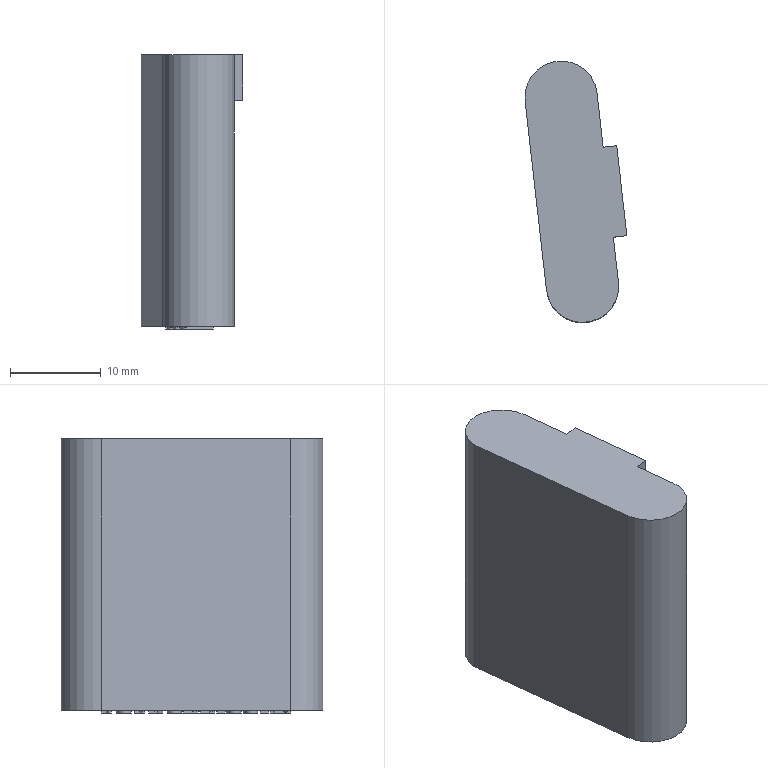Part | NX | features 13 2 | 1 solid | 113 faces | box 11.265 x 28.872 x 30.3 mm | volume 6630 mm3 | plane 94 | spline 17 | cylinder 2 | commonest cylinder face diameters 8 x2